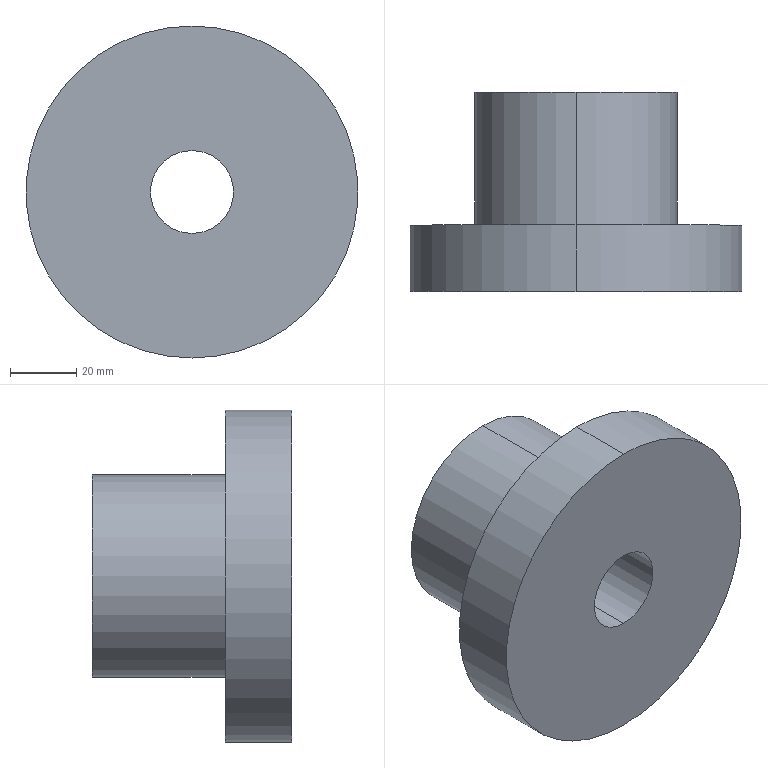Part | SolidWorks | features Revolution 1 | 1 solid | 12 faces | box 100 x 60 x 100 mm | volume 182448 mm3 | cylinder 8 | plane 4 | commonest cylinder face diameters 25 x2 51 x2 61 x2 100 x2
STEP:
#1=CARTESIAN_POINT('',(0.,60.,-30.5));
#2=VERTEX_POINT('',#1);
#3=CARTESIAN_POINT('',(0.,60.,30.5));
#4=VERTEX_POINT('',#3);
#5=CARTESIAN_POINT('',(0.,60.,0.));
#6=DIRECTION('',(0.,-1.,0.));
#7=DIRECTION('',(0.,0.,-1.));
#8=AXIS2_PLACEMENT_3D('',#5,#6,#7);
#9=CIRCLE('',#8,30.5);
#10=EDGE_CURVE('',#2,#4,#9,.T.);
#11=ORIENTED_EDGE('',*,*,#10,.T.);
#12=CARTESIAN_POINT('',(0.,20.,30.5));
#13=VERTEX_POINT('',#12);
#14=CARTESIAN_POINT('',(0.,0.,30.5));
#15=DIRECTION('',(0.,-1.,0.));
#16=VECTOR('',#15,1000.);
#17=LINE('',#14,#16);
#18=EDGE_CURVE('',#4,#13,#17,.T.);
#19=ORIENTED_EDGE('',*,*,#18,.T.);
#20=CARTESIAN_POINT('',(0.,20.,-30.5));
#21=VERTEX_POINT('',#20);
#22=CARTESIAN_POINT('',(0.,20.,0.));
#23=DIRECTION('',(0.,-1.,0.));
#24=DIRECTION('',(0.,0.,-1.));
#25=AXIS2_PLACEMENT_3D('',#22,#23,#24);
#26=CIRCLE('',#25,30.5);
#27=EDGE_CURVE('',#21,#13,#26,.T.);
#28=ORIENTED_EDGE('',*,*,#27,.F.);
#29=CARTESIAN_POINT('',(0.,0.,-30.5));
#30=DIRECTION('',(0.,-1.,0.));
#31=VECTOR('',#30,1000.);
#32=LINE('',#29,#31);
#33=EDGE_CURVE('',#2,#21,#32,.T.);
#34=ORIENTED_EDGE('',*,*,#33,.F.);
#35=EDGE_LOOP('',(#11,#19,#28,#34));
#36=FACE_OUTER_BOUND('',#35,.T.);
#37=CARTESIAN_POINT('',(0.,0.,0.));
#38=DIRECTION('',(0.,-1.,0.));
#39=DIRECTION('',(0.,0.,-1.));
#40=AXIS2_PLACEMENT_3D('',#37,#38,#39);
#41=CYLINDRICAL_SURFACE('',#40,30.5);
#42=ADVANCED_FACE('',(#36),#41,.T.);
#43=CARTESIAN_POINT('',(0.,20.,-50.));
#44=VERTEX_POINT('',#43);
#45=CARTESIAN_POINT('',(0.,20.,50.));
#46=VERTEX_POINT('',#45);
#47=CARTESIAN_POINT('',(0.,20.,0.));
#48=DIRECTION('',(0.,-1.,0.));
#49=DIRECTION('',(0.,0.,-1.));
#50=AXIS2_PLACEMENT_3D('',#47,#48,#49);
#51=CIRCLE('',#50,50.);
#52=EDGE_CURVE('',#44,#46,#51,.T.);
#53=ORIENTED_EDGE('',*,*,#52,.T.);
#54=CARTESIAN_POINT('',(0.,0.,50.));
#55=VERTEX_POINT('',#54);
#56=CARTESIAN_POINT('',(0.,0.,50.));
#57=DIRECTION('',(0.,-1.,0.));
#58=VECTOR('',#57,1000.);
#59=LINE('',#56,#58);
#60=EDGE_CURVE('',#46,#55,#59,.T.);
#61=ORIENTED_EDGE('',*,*,#60,.T.);
#62=CARTESIAN_POINT('',(0.,0.,-50.));
#63=VERTEX_POINT('',#62);
#64=CARTESIAN_POINT('',(0.,0.,0.));
#65=DIRECTION('',(0.,-1.,0.));
#66=DIRECTION('',(0.,0.,-1.));
#67=AXIS2_PLACEMENT_3D('',#64,#65,#66);
#68=CIRCLE('',#67,50.);
#69=EDGE_CURVE('',#63,#55,#68,.T.);
#70=ORIENTED_EDGE('',*,*,#69,.F.);
#71=CARTESIAN_POINT('',(0.,0.,-50.));
#72=DIRECTION('',(0.,-1.,0.));
#73=VECTOR('',#72,1000.);
#74=LINE('',#71,#73);
#75=EDGE_CURVE('',#44,#63,#74,.T.);
#76=ORIENTED_EDGE('',*,*,#75,.F.);
#77=EDGE_LOOP('',(#53,#61,#70,#76));
#78=FACE_OUTER_BOUND('',#77,.T.);
#79=CARTESIAN_POINT('',(0.,0.,0.));
#80=DIRECTION('',(0.,-1.,0.));
#81=DIRECTION('',(0.,0.,-1.));
#82=AXIS2_PLACEMENT_3D('',#79,#80,#81);
#83=CYLINDRICAL_SURFACE('',#82,50.);
#84=ADVANCED_FACE('',(#78),#83,.T.);
#85=CARTESIAN_POINT('',(0.,20.,12.5));
#86=VERTEX_POINT('',#85);
#87=CARTESIAN_POINT('',(0.,20.,-12.5));
#88=VERTEX_POINT('',#87);
#89=CARTESIAN_POINT('',(0.,20.,0.));
#90=DIRECTION('',(0.,-1.,0.));
#91=DIRECTION('',(0.,0.,-1.));
#92=AXIS2_PLACEMENT_3D('',#89,#90,#91);
#93=CIRCLE('',#92,12.5);
#94=EDGE_CURVE('',#86,#88,#93,.T.);
#95=ORIENTED_EDGE('',*,*,#94,.F.);
#96=CARTESIAN_POINT('',(0.,0.,12.5));
#97=VERTEX_POINT('',#96);
#98=CARTESIAN_POINT('',(0.,0.,12.5));
#99=DIRECTION('',(0.,-1.,0.));
#100=VECTOR('',#99,1000.);
#101=LINE('',#98,#100);
#102=EDGE_CURVE('',#86,#97,#101,.T.);
#103=ORIENTED_EDGE('',*,*,#102,.T.);
#104=CARTESIAN_POINT('',(0.,0.,-12.5));
#105=VERTEX_POINT('',#104);
#106=CARTESIAN_POINT('',(0.,0.,0.));
#107=DIRECTION('',(0.,-1.,0.));
#108=DIRECTION('',(0.,0.,-1.));
#109=AXIS2_PLACEMENT_3D('',#106,#107,#108);
#110=CIRCLE('',#109,12.5);
#111=EDGE_CURVE('',#97,#105,#110,.T.);
#112=ORIENTED_EDGE('',*,*,#111,.T.);
#113=CARTESIAN_POINT('',(0.,0.,-12.5));
#114=DIRECTION('',(0.,-1.,0.));
#115=VECTOR('',#114,1000.);
#116=LINE('',#113,#115);
#117=EDGE_CURVE('',#88,#105,#116,.T.);
#118=ORIENTED_EDGE('',*,*,#117,.F.);
#119=EDGE_LOOP('',(#95,#103,#112,#118));
#120=FACE_OUTER_BOUND('',#119,.T.);
#121=CARTESIAN_POINT('',(0.,0.,0.));
#122=DIRECTION('',(0.,-1.,0.));
#123=DIRECTION('',(0.,0.,-1.));
#124=AXIS2_PLACEMENT_3D('',#121,#122,#123);
#125=CYLINDRICAL_SURFACE('',#124,12.5);
#126=ADVANCED_FACE('',(#120),#125,.F.);
#127=CARTESIAN_POINT('',(0.,60.,25.5));
#128=VERTEX_POINT('',#127);
#129=CARTESIAN_POINT('',(0.,60.,-25.5));
#130=VERTEX_POINT('',#129);
#131=CARTESIAN_POINT('',(0.,60.,0.));
#132=DIRECTION('',(0.,-1.,0.));
#133=DIRECTION('',(0.,0.,-1.));
#134=AXIS2_PLACEMENT_3D('',#131,#132,#133);
#135=CIRCLE('',#134,25.5);
#136=EDGE_CURVE('',#128,#130,#135,.T.);
#137=ORIENTED_EDGE('',*,*,#136,.F.);
#138=CARTESIAN_POINT('',(0.,20.,25.5));
#139=VERTEX_POINT('',#138);
#140=CARTESIAN_POINT('',(0.,0.,25.5));
#141=DIRECTION('',(0.,-1.,0.));
#142=VECTOR('',#141,1000.);
#143=LINE('',#140,#142);
#144=EDGE_CURVE('',#128,#139,#143,.T.);
#145=ORIENTED_EDGE('',*,*,#144,.T.);
#146=CARTESIAN_POINT('',(0.,20.,-25.5));
#147=VERTEX_POINT('',#146);
#148=CARTESIAN_POINT('',(0.,20.,0.));
#149=DIRECTION('',(0.,-1.,0.));
#150=DIRECTION('',(0.,0.,-1.));
#151=AXIS2_PLACEMENT_3D('',#148,#149,#150);
#152=CIRCLE('',#151,25.5);
#153=EDGE_CURVE('',#139,#147,#152,.T.);
#154=ORIENTED_EDGE('',*,*,#153,.T.);
#155=CARTESIAN_POINT('',(0.,0.,-25.5));
#156=DIRECTION('',(0.,-1.,0.));
#157=VECTOR('',#156,1000.);
#158=LINE('',#155,#157);
#159=EDGE_CURVE('',#130,#147,#158,.T.);
#160=ORIENTED_EDGE('',*,*,#159,.F.);
#161=EDGE_LOOP('',(#137,#145,#154,#160));
#162=FACE_OUTER_BOUND('',#161,.T.);
#163=CARTESIAN_POINT('',(0.,0.,0.));
#164=DIRECTION('',(0.,-1.,0.));
#165=DIRECTION('',(0.,0.,-1.));
#166=AXIS2_PLACEMENT_3D('',#163,#164,#165);
#167=CYLINDRICAL_SURFACE('',#166,25.5);
#168=ADVANCED_FACE('',(#162),#167,.F.);
#169=CARTESIAN_POINT('',(0.,60.,0.));
#170=DIRECTION('',(0.,-1.,0.));
#171=DIRECTION('',(0.,0.,-1.));
#172=AXIS2_PLACEMENT_3D('',#169,#170,#171);
#173=CIRCLE('',#172,25.5);
#174=EDGE_CURVE('',#130,#128,#173,.T.);
#175=ORIENTED_EDGE('',*,*,#174,.T.);
#176=ORIENTED_EDGE('',*,*,#136,.T.);
#177=EDGE_LOOP('',(#175,#176));
#178=FACE_BOUND('',#177,.T.);
#179=ORIENTED_EDGE('',*,*,#10,.F.);
#180=CARTESIAN_POINT('',(0.,60.,0.));
#181=DIRECTION('',(0.,-1.,0.));
#182=DIRECTION('',(0.,0.,-1.));
#183=AXIS2_PLACEMENT_3D('',#180,#181,#182);
#184=CIRCLE('',#183,30.5);
#185=EDGE_CURVE('',#4,#2,#184,.T.);
#186=ORIENTED_EDGE('',*,*,#185,.F.);
#187=EDGE_LOOP('',(#179,#186));
#188=FACE_OUTER_BOUND('',#187,.T.);
#189=CARTESIAN_POINT('',(30.5,60.,0.));
#190=DIRECTION('',(0.,1.,0.));
#191=DIRECTION('',(0.,0.,1.));
#192=AXIS2_PLACEMENT_3D('',#189,#190,#191);
#193=PLANE('',#192);
#194=ADVANCED_FACE('',(#178,#188),#193,.T.);
#195=ORIENTED_EDGE('',*,*,#144,.F.);
#196=ORIENTED_EDGE('',*,*,#174,.F.);
#197=ORIENTED_EDGE('',*,*,#159,.T.);
#198=CARTESIAN_POINT('',(0.,20.,0.));
#199=DIRECTION('',(0.,-1.,0.));
#200=DIRECTION('',(0.,0.,-1.));
#201=AXIS2_PLACEMENT_3D('',#198,#199,#200);
#202=CIRCLE('',#201,25.5);
#203=EDGE_CURVE('',#147,#139,#202,.T.);
#204=ORIENTED_EDGE('',*,*,#203,.T.);
#205=EDGE_LOOP('',(#195,#196,#197,#204));
#206=FACE_OUTER_BOUND('',#205,.T.);
#207=CARTESIAN_POINT('',(0.,0.,0.));
#208=DIRECTION('',(0.,-1.,0.));
#209=DIRECTION('',(0.,0.,-1.));
#210=AXIS2_PLACEMENT_3D('',#207,#208,#209);
#211=CYLINDRICAL_SURFACE('',#210,25.5);
#212=ADVANCED_FACE('',(#206),#211,.F.);
#213=CARTESIAN_POINT('',(0.,20.,0.));
#214=DIRECTION('',(0.,-1.,0.));
#215=DIRECTION('',(0.,0.,-1.));
#216=AXIS2_PLACEMENT_3D('',#213,#214,#215);
#217=CIRCLE('',#216,12.5);
#218=EDGE_CURVE('',#88,#86,#217,.T.);
#219=ORIENTED_EDGE('',*,*,#218,.T.);
#220=ORIENTED_EDGE('',*,*,#94,.T.);
#221=EDGE_LOOP('',(#219,#220));
#222=FACE_BOUND('',#221,.T.);
#223=ORIENTED_EDGE('',*,*,#203,.F.);
#224=ORIENTED_EDGE('',*,*,#153,.F.);
#225=EDGE_LOOP('',(#223,#224));
#226=FACE_OUTER_BOUND('',#225,.T.);
#227=CARTESIAN_POINT('',(25.5,20.,0.));
#228=DIRECTION('',(0.,1.,0.));
#229=DIRECTION('',(0.,0.,1.));
#230=AXIS2_PLACEMENT_3D('',#227,#228,#229);
#231=PLANE('',#230);
#232=ADVANCED_FACE('',(#222,#226),#231,.T.);
#233=ORIENTED_EDGE('',*,*,#102,.F.);
#234=ORIENTED_EDGE('',*,*,#218,.F.);
#235=ORIENTED_EDGE('',*,*,#117,.T.);
#236=CARTESIAN_POINT('',(0.,0.,0.));
#237=DIRECTION('',(0.,-1.,0.));
#238=DIRECTION('',(0.,0.,-1.));
#239=AXIS2_PLACEMENT_3D('',#236,#237,#238);
#240=CIRCLE('',#239,12.5);
#241=EDGE_CURVE('',#105,#97,#240,.T.);
#242=ORIENTED_EDGE('',*,*,#241,.T.);
#243=EDGE_LOOP('',(#233,#234,#235,#242));
#244=FACE_OUTER_BOUND('',#243,.T.);
#245=CARTESIAN_POINT('',(0.,0.,0.));
#246=DIRECTION('',(0.,-1.,0.));
#247=DIRECTION('',(0.,0.,-1.));
#248=AXIS2_PLACEMENT_3D('',#245,#246,#247);
#249=CYLINDRICAL_SURFACE('',#248,12.5);
#250=ADVANCED_FACE('',(#244),#249,.F.);
#251=ORIENTED_EDGE('',*,*,#69,.T.);
#252=CARTESIAN_POINT('',(0.,0.,0.));
#253=DIRECTION('',(0.,-1.,0.));
#254=DIRECTION('',(0.,0.,-1.));
#255=AXIS2_PLACEMENT_3D('',#252,#253,#254);
#256=CIRCLE('',#255,50.);
#257=EDGE_CURVE('',#55,#63,#256,.T.);
#258=ORIENTED_EDGE('',*,*,#257,.T.);
#259=EDGE_LOOP('',(#251,#258));
#260=FACE_OUTER_BOUND('',#259,.T.);
#261=ORIENTED_EDGE('',*,*,#241,.F.);
#262=ORIENTED_EDGE('',*,*,#111,.F.);
#263=EDGE_LOOP('',(#261,#262));
#264=FACE_BOUND('',#263,.T.);
#265=CARTESIAN_POINT('',(12.5,0.,0.));
#266=DIRECTION('',(0.,-1.,0.));
#267=DIRECTION('',(0.,0.,-1.));
#268=AXIS2_PLACEMENT_3D('',#265,#266,#267);
#269=PLANE('',#268);
#270=ADVANCED_FACE('',(#260,#264),#269,.T.);
#271=ORIENTED_EDGE('',*,*,#60,.F.);
#272=CARTESIAN_POINT('',(0.,20.,0.));
#273=DIRECTION('',(0.,-1.,0.));
#274=DIRECTION('',(0.,0.,-1.));
#275=AXIS2_PLACEMENT_3D('',#272,#273,#274);
#276=CIRCLE('',#275,50.);
#277=EDGE_CURVE('',#46,#44,#276,.T.);
#278=ORIENTED_EDGE('',*,*,#277,.T.);
#279=ORIENTED_EDGE('',*,*,#75,.T.);
#280=ORIENTED_EDGE('',*,*,#257,.F.);
#281=EDGE_LOOP('',(#271,#278,#279,#280));
#282=FACE_OUTER_BOUND('',#281,.T.);
#283=CARTESIAN_POINT('',(0.,0.,0.));
#284=DIRECTION('',(0.,-1.,0.));
#285=DIRECTION('',(0.,0.,-1.));
#286=AXIS2_PLACEMENT_3D('',#283,#284,#285);
#287=CYLINDRICAL_SURFACE('',#286,50.);
#288=ADVANCED_FACE('',(#282),#287,.T.);
#289=ORIENTED_EDGE('',*,*,#27,.T.);
#290=CARTESIAN_POINT('',(0.,20.,0.));
#291=DIRECTION('',(0.,-1.,0.));
#292=DIRECTION('',(0.,0.,-1.));
#293=AXIS2_PLACEMENT_3D('',#290,#291,#292);
#294=CIRCLE('',#293,30.5);
#295=EDGE_CURVE('',#13,#21,#294,.T.);
#296=ORIENTED_EDGE('',*,*,#295,.T.);
#297=EDGE_LOOP('',(#289,#296));
#298=FACE_BOUND('',#297,.T.);
#299=ORIENTED_EDGE('',*,*,#52,.F.);
#300=ORIENTED_EDGE('',*,*,#277,.F.);
#301=EDGE_LOOP('',(#299,#300));
#302=FACE_OUTER_BOUND('',#301,.T.);
#303=CARTESIAN_POINT('',(50.,20.,0.));
#304=DIRECTION('',(0.,1.,0.));
#305=DIRECTION('',(0.,0.,1.));
#306=AXIS2_PLACEMENT_3D('',#303,#304,#305);
#307=PLANE('',#306);
#308=ADVANCED_FACE('',(#298,#302),#307,.T.);
#309=ORIENTED_EDGE('',*,*,#18,.F.);
#310=ORIENTED_EDGE('',*,*,#185,.T.);
#311=ORIENTED_EDGE('',*,*,#33,.T.);
#312=ORIENTED_EDGE('',*,*,#295,.F.);
#313=EDGE_LOOP('',(#309,#310,#311,#312));
#314=FACE_OUTER_BOUND('',#313,.T.);
#315=CARTESIAN_POINT('',(0.,0.,0.));
#316=DIRECTION('',(0.,-1.,0.));
#317=DIRECTION('',(0.,0.,-1.));
#318=AXIS2_PLACEMENT_3D('',#315,#316,#317);
#319=CYLINDRICAL_SURFACE('',#318,30.5);
#320=ADVANCED_FACE('',(#314),#319,.T.);
#321=CLOSED_SHELL('',(#42,#84,#126,#168,#194,#212,#232,#250,#270,#288,#308,#320));
#322=MANIFOLD_SOLID_BREP('',#321);
#323=CARTESIAN_POINT('',(0.,0.,0.));
#324=DIRECTION('',(0.,0.,1.));
#325=DIRECTION('',(1.,0.,0.));
#326=AXIS2_PLACEMENT_3D('',#323,#324,#325);
#327=(LENGTH_UNIT()NAMED_UNIT(*)SI_UNIT(.MILLI.,.METRE.));
#328=UNCERTAINTY_MEASURE_WITH_UNIT(LENGTH_MEASURE(0.00001),#327,'','');
#329=(NAMED_UNIT(*)PLANE_ANGLE_UNIT()SI_UNIT($,.RADIAN.));
#330=(NAMED_UNIT(*)SI_UNIT($,.STERADIAN.)SOLID_ANGLE_UNIT());
#331=(GEOMETRIC_REPRESENTATION_CONTEXT(3)GLOBAL_UNCERTAINTY_ASSIGNED_CONTEXT((#328))GLOBAL_UNIT_ASSIGNED_CONTEXT((#327,#329,#330))REPRESENTATION_CONTEXT('',''));
#332=ADVANCED_BREP_SHAPE_REPRESENTATION('',(#322,#326),#331);